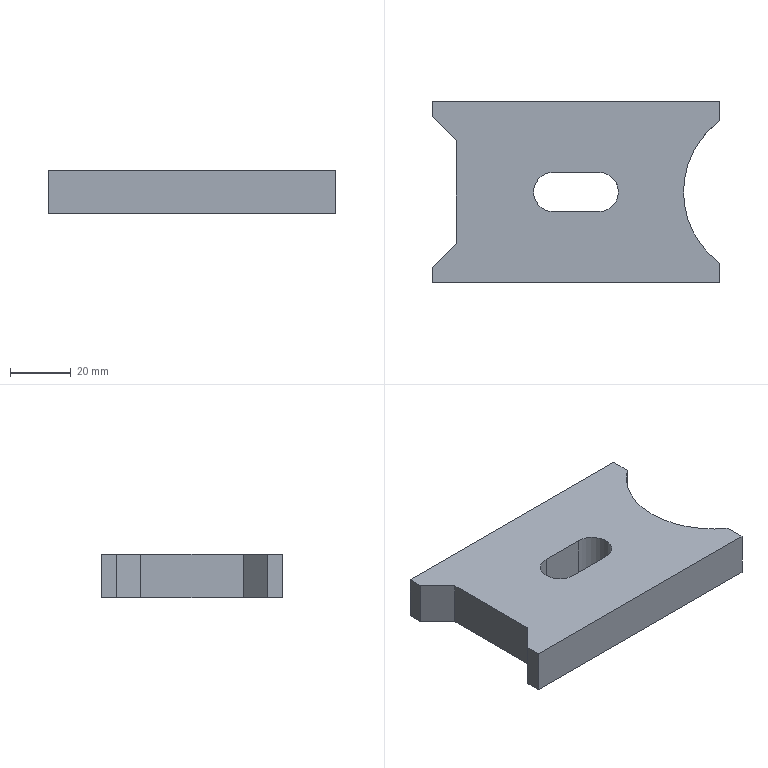Part | SolidWorks | features ICE 2, Shell 2, Extrusion 1 | 1 solid | 18 faces | box 95 x 60 x 14.5 mm | volume 67299 mm3 | plane 13 | cylinder 5 | commonest cylinder face diameters 13 x3 58.021 x2
STEP:
#1=CARTESIAN_POINT('',(47.5,23.5,14.5));
#2=VERTEX_POINT('',#1);
#3=CARTESIAN_POINT('',(35.5,0.,14.5));
#4=VERTEX_POINT('',#3);
#5=CARTESIAN_POINT('',(64.51,0.,14.5));
#6=DIRECTION('',(0.,0.,1.));
#7=DIRECTION('',(1.,0.,0.));
#8=AXIS2_PLACEMENT_3D('',#5,#6,#7);
#9=CIRCLE('',#8,29.01);
#10=EDGE_CURVE('',#2,#4,#9,.T.);
#11=ORIENTED_EDGE('',*,*,#10,.T.);
#12=CARTESIAN_POINT('',(35.5,0.,0.));
#13=VERTEX_POINT('',#12);
#14=CARTESIAN_POINT('',(35.5,0.,14.5));
#15=DIRECTION('',(0.,0.,-1.));
#16=VECTOR('',#15,1000.);
#17=LINE('',#14,#16);
#18=EDGE_CURVE('',#4,#13,#17,.T.);
#19=ORIENTED_EDGE('',*,*,#18,.T.);
#20=CARTESIAN_POINT('',(47.5,23.5,0.));
#21=VERTEX_POINT('',#20);
#22=CARTESIAN_POINT('',(64.51,0.,0.));
#23=DIRECTION('',(0.,0.,1.));
#24=DIRECTION('',(1.,0.,0.));
#25=AXIS2_PLACEMENT_3D('',#22,#23,#24);
#26=CIRCLE('',#25,29.01);
#27=EDGE_CURVE('',#21,#13,#26,.T.);
#28=ORIENTED_EDGE('',*,*,#27,.F.);
#29=CARTESIAN_POINT('',(47.5,23.5,14.5));
#30=DIRECTION('',(0.,0.,-1.));
#31=VECTOR('',#30,1000.);
#32=LINE('',#29,#31);
#33=EDGE_CURVE('',#2,#21,#32,.T.);
#34=ORIENTED_EDGE('',*,*,#33,.F.);
#35=EDGE_LOOP('',(#11,#19,#28,#34));
#36=FACE_OUTER_BOUND('',#35,.T.);
#37=CARTESIAN_POINT('',(64.51,0.,14.5));
#38=DIRECTION('',(0.,0.,-1.));
#39=DIRECTION('',(-1.,0.,0.));
#40=AXIS2_PLACEMENT_3D('',#37,#38,#39);
#41=CYLINDRICAL_SURFACE('',#40,29.01);
#42=ADVANCED_FACE('',(#36),#41,.F.);
#43=CARTESIAN_POINT('',(-14.,0.,14.5));
#44=VERTEX_POINT('',#43);
#45=CARTESIAN_POINT('',(-7.5,6.5,14.5));
#46=VERTEX_POINT('',#45);
#47=CARTESIAN_POINT('',(-7.5,0.,14.5));
#48=DIRECTION('',(0.,0.,-1.));
#49=DIRECTION('',(1.,0.,0.));
#50=AXIS2_PLACEMENT_3D('',#47,#48,#49);
#51=CIRCLE('',#50,6.5);
#52=EDGE_CURVE('',#44,#46,#51,.T.);
#53=ORIENTED_EDGE('',*,*,#52,.F.);
#54=CARTESIAN_POINT('',(-14.,0.,0.));
#55=VERTEX_POINT('',#54);
#56=CARTESIAN_POINT('',(-14.,0.,14.5));
#57=DIRECTION('',(0.,0.,-1.));
#58=VECTOR('',#57,1000.);
#59=LINE('',#56,#58);
#60=EDGE_CURVE('',#44,#55,#59,.T.);
#61=ORIENTED_EDGE('',*,*,#60,.T.);
#62=CARTESIAN_POINT('',(-7.5,6.5,0.));
#63=VERTEX_POINT('',#62);
#64=CARTESIAN_POINT('',(-7.5,0.,0.));
#65=DIRECTION('',(0.,0.,-1.));
#66=DIRECTION('',(1.,0.,0.));
#67=AXIS2_PLACEMENT_3D('',#64,#65,#66);
#68=CIRCLE('',#67,6.5);
#69=EDGE_CURVE('',#55,#63,#68,.T.);
#70=ORIENTED_EDGE('',*,*,#69,.T.);
#71=CARTESIAN_POINT('',(-7.5,6.5,14.5));
#72=DIRECTION('',(0.,0.,-1.));
#73=VECTOR('',#72,1000.);
#74=LINE('',#71,#73);
#75=EDGE_CURVE('',#46,#63,#74,.T.);
#76=ORIENTED_EDGE('',*,*,#75,.F.);
#77=EDGE_LOOP('',(#53,#61,#70,#76));
#78=FACE_OUTER_BOUND('',#77,.T.);
#79=CARTESIAN_POINT('',(-7.5,0.,14.5));
#80=DIRECTION('',(0.,0.,-1.));
#81=DIRECTION('',(-1.,0.,0.));
#82=AXIS2_PLACEMENT_3D('',#79,#80,#81);
#83=CYLINDRICAL_SURFACE('',#82,6.5);
#84=ADVANCED_FACE('',(#78),#83,.F.);
#85=CARTESIAN_POINT('',(-7.5,-6.5,0.));
#86=VERTEX_POINT('',#85);
#87=CARTESIAN_POINT('',(7.5,-6.5,0.));
#88=VERTEX_POINT('',#87);
#89=CARTESIAN_POINT('',(0.,-6.5,0.));
#90=DIRECTION('',(1.,0.,0.));
#91=VECTOR('',#90,1000.);
#92=LINE('',#89,#91);
#93=EDGE_CURVE('',#86,#88,#92,.T.);
#94=ORIENTED_EDGE('',*,*,#93,.F.);
#95=CARTESIAN_POINT('',(-7.5,-6.5,14.5));
#96=VERTEX_POINT('',#95);
#97=CARTESIAN_POINT('',(-7.5,-6.5,14.5));
#98=DIRECTION('',(0.,0.,-1.));
#99=VECTOR('',#98,1000.);
#100=LINE('',#97,#99);
#101=EDGE_CURVE('',#96,#86,#100,.T.);
#102=ORIENTED_EDGE('',*,*,#101,.F.);
#103=CARTESIAN_POINT('',(7.5,-6.5,14.5));
#104=VERTEX_POINT('',#103);
#105=CARTESIAN_POINT('',(0.,-6.5,14.5));
#106=DIRECTION('',(1.,0.,0.));
#107=VECTOR('',#106,1000.);
#108=LINE('',#105,#107);
#109=EDGE_CURVE('',#96,#104,#108,.T.);
#110=ORIENTED_EDGE('',*,*,#109,.T.);
#111=CARTESIAN_POINT('',(7.5,-6.5,14.5));
#112=DIRECTION('',(0.,0.,-1.));
#113=VECTOR('',#112,1000.);
#114=LINE('',#111,#113);
#115=EDGE_CURVE('',#104,#88,#114,.T.);
#116=ORIENTED_EDGE('',*,*,#115,.T.);
#117=EDGE_LOOP('',(#94,#102,#110,#116));
#118=FACE_OUTER_BOUND('',#117,.T.);
#119=CARTESIAN_POINT('',(0.,-6.5,14.5));
#120=DIRECTION('',(0.,1.,0.));
#121=DIRECTION('',(-1.,0.,0.));
#122=AXIS2_PLACEMENT_3D('',#119,#120,#121);
#123=PLANE('',#122);
#124=ADVANCED_FACE('',(#118),#123,.T.);
#125=ORIENTED_EDGE('',*,*,#60,.F.);
#126=CARTESIAN_POINT('',(-7.5,0.,14.5));
#127=DIRECTION('',(0.,0.,-1.));
#128=DIRECTION('',(1.,0.,0.));
#129=AXIS2_PLACEMENT_3D('',#126,#127,#128);
#130=CIRCLE('',#129,6.5);
#131=EDGE_CURVE('',#96,#44,#130,.T.);
#132=ORIENTED_EDGE('',*,*,#131,.F.);
#133=ORIENTED_EDGE('',*,*,#101,.T.);
#134=CARTESIAN_POINT('',(-7.5,0.,0.));
#135=DIRECTION('',(0.,0.,-1.));
#136=DIRECTION('',(1.,0.,0.));
#137=AXIS2_PLACEMENT_3D('',#134,#135,#136);
#138=CIRCLE('',#137,6.5);
#139=EDGE_CURVE('',#86,#55,#138,.T.);
#140=ORIENTED_EDGE('',*,*,#139,.T.);
#141=EDGE_LOOP('',(#125,#132,#133,#140));
#142=FACE_OUTER_BOUND('',#141,.T.);
#143=CARTESIAN_POINT('',(-7.5,0.,14.5));
#144=DIRECTION('',(0.,0.,-1.));
#145=DIRECTION('',(-1.,0.,0.));
#146=AXIS2_PLACEMENT_3D('',#143,#144,#145);
#147=CYLINDRICAL_SURFACE('',#146,6.5);
#148=ADVANCED_FACE('',(#142),#147,.F.);
#149=CARTESIAN_POINT('',(7.5,6.5,0.));
#150=VERTEX_POINT('',#149);
#151=CARTESIAN_POINT('',(0.,6.5,0.));
#152=DIRECTION('',(1.,0.,0.));
#153=VECTOR('',#152,1000.);
#154=LINE('',#151,#153);
#155=EDGE_CURVE('',#63,#150,#154,.T.);
#156=ORIENTED_EDGE('',*,*,#155,.T.);
#157=CARTESIAN_POINT('',(7.5,6.5,14.5));
#158=VERTEX_POINT('',#157);
#159=CARTESIAN_POINT('',(7.5,6.5,14.5));
#160=DIRECTION('',(0.,0.,-1.));
#161=VECTOR('',#160,1000.);
#162=LINE('',#159,#161);
#163=EDGE_CURVE('',#158,#150,#162,.T.);
#164=ORIENTED_EDGE('',*,*,#163,.F.);
#165=CARTESIAN_POINT('',(0.,6.5,14.5));
#166=DIRECTION('',(1.,0.,0.));
#167=VECTOR('',#166,1000.);
#168=LINE('',#165,#167);
#169=EDGE_CURVE('',#46,#158,#168,.T.);
#170=ORIENTED_EDGE('',*,*,#169,.F.);
#171=ORIENTED_EDGE('',*,*,#75,.T.);
#172=EDGE_LOOP('',(#156,#164,#170,#171));
#173=FACE_OUTER_BOUND('',#172,.T.);
#174=CARTESIAN_POINT('',(0.,6.5,14.5));
#175=DIRECTION('',(0.,1.,0.));
#176=DIRECTION('',(-1.,0.,0.));
#177=AXIS2_PLACEMENT_3D('',#174,#175,#176);
#178=PLANE('',#177);
#179=ADVANCED_FACE('',(#173),#178,.F.);
#180=ORIENTED_EDGE('',*,*,#18,.F.);
#181=CARTESIAN_POINT('',(47.5,-23.5,14.5));
#182=VERTEX_POINT('',#181);
#183=CARTESIAN_POINT('',(64.51,0.,14.5));
#184=DIRECTION('',(0.,0.,1.));
#185=DIRECTION('',(1.,0.,0.));
#186=AXIS2_PLACEMENT_3D('',#183,#184,#185);
#187=CIRCLE('',#186,29.01);
#188=EDGE_CURVE('',#4,#182,#187,.T.);
#189=ORIENTED_EDGE('',*,*,#188,.T.);
#190=CARTESIAN_POINT('',(47.5,-23.5,0.));
#191=VERTEX_POINT('',#190);
#192=CARTESIAN_POINT('',(47.5,-23.5,14.5));
#193=DIRECTION('',(0.,0.,-1.));
#194=VECTOR('',#193,1000.);
#195=LINE('',#192,#194);
#196=EDGE_CURVE('',#182,#191,#195,.T.);
#197=ORIENTED_EDGE('',*,*,#196,.T.);
#198=CARTESIAN_POINT('',(64.51,0.,0.));
#199=DIRECTION('',(0.,0.,1.));
#200=DIRECTION('',(1.,0.,0.));
#201=AXIS2_PLACEMENT_3D('',#198,#199,#200);
#202=CIRCLE('',#201,29.01);
#203=EDGE_CURVE('',#13,#191,#202,.T.);
#204=ORIENTED_EDGE('',*,*,#203,.F.);
#205=EDGE_LOOP('',(#180,#189,#197,#204));
#206=FACE_OUTER_BOUND('',#205,.T.);
#207=CARTESIAN_POINT('',(64.51,0.,14.5));
#208=DIRECTION('',(0.,0.,-1.));
#209=DIRECTION('',(-1.,0.,0.));
#210=AXIS2_PLACEMENT_3D('',#207,#208,#209);
#211=CYLINDRICAL_SURFACE('',#210,29.01);
#212=ADVANCED_FACE('',(#206),#211,.F.);
#213=CARTESIAN_POINT('',(47.5,30.,0.));
#214=VERTEX_POINT('',#213);
#215=CARTESIAN_POINT('',(47.5,0.,0.));
#216=DIRECTION('',(0.,-1.,0.));
#217=VECTOR('',#216,1000.);
#218=LINE('',#215,#217);
#219=EDGE_CURVE('',#214,#21,#218,.T.);
#220=ORIENTED_EDGE('',*,*,#219,.F.);
#221=CARTESIAN_POINT('',(47.5,30.,14.5));
#222=VERTEX_POINT('',#221);
#223=CARTESIAN_POINT('',(47.5,30.,14.5));
#224=DIRECTION('',(0.,0.,-1.));
#225=VECTOR('',#224,1000.);
#226=LINE('',#223,#225);
#227=EDGE_CURVE('',#222,#214,#226,.T.);
#228=ORIENTED_EDGE('',*,*,#227,.F.);
#229=CARTESIAN_POINT('',(47.5,0.,14.5));
#230=DIRECTION('',(0.,-1.,0.));
#231=VECTOR('',#230,1000.);
#232=LINE('',#229,#231);
#233=EDGE_CURVE('',#222,#2,#232,.T.);
#234=ORIENTED_EDGE('',*,*,#233,.T.);
#235=ORIENTED_EDGE('',*,*,#33,.T.);
#236=EDGE_LOOP('',(#220,#228,#234,#235));
#237=FACE_OUTER_BOUND('',#236,.T.);
#238=CARTESIAN_POINT('',(47.5,0.,14.5));
#239=DIRECTION('',(1.,0.,0.));
#240=DIRECTION('',(0.,1.,0.));
#241=AXIS2_PLACEMENT_3D('',#238,#239,#240);
#242=PLANE('',#241);
#243=ADVANCED_FACE('',(#237),#242,.T.);
#244=CARTESIAN_POINT('',(-47.5,30.,0.));
#245=VERTEX_POINT('',#244);
#246=CARTESIAN_POINT('',(0.,30.,0.));
#247=DIRECTION('',(1.,0.,0.));
#248=VECTOR('',#247,1000.);
#249=LINE('',#246,#248);
#250=EDGE_CURVE('',#245,#214,#249,.T.);
#251=ORIENTED_EDGE('',*,*,#250,.F.);
#252=CARTESIAN_POINT('',(-47.5,30.,14.5));
#253=VERTEX_POINT('',#252);
#254=CARTESIAN_POINT('',(-47.5,30.,14.5));
#255=DIRECTION('',(0.,0.,-1.));
#256=VECTOR('',#255,1000.);
#257=LINE('',#254,#256);
#258=EDGE_CURVE('',#253,#245,#257,.T.);
#259=ORIENTED_EDGE('',*,*,#258,.F.);
#260=CARTESIAN_POINT('',(0.,30.,14.5));
#261=DIRECTION('',(1.,0.,0.));
#262=VECTOR('',#261,1000.);
#263=LINE('',#260,#262);
#264=EDGE_CURVE('',#253,#222,#263,.T.);
#265=ORIENTED_EDGE('',*,*,#264,.T.);
#266=ORIENTED_EDGE('',*,*,#227,.T.);
#267=EDGE_LOOP('',(#251,#259,#265,#266));
#268=FACE_OUTER_BOUND('',#267,.T.);
#269=CARTESIAN_POINT('',(0.,30.,14.5));
#270=DIRECTION('',(0.,1.,0.));
#271=DIRECTION('',(0.,0.,1.));
#272=AXIS2_PLACEMENT_3D('',#269,#270,#271);
#273=PLANE('',#272);
#274=ADVANCED_FACE('',(#268),#273,.T.);
#275=CARTESIAN_POINT('',(-47.5,25.,0.));
#276=VERTEX_POINT('',#275);
#277=CARTESIAN_POINT('',(-47.5,0.,0.));
#278=DIRECTION('',(0.,-1.,0.));
#279=VECTOR('',#278,1000.);
#280=LINE('',#277,#279);
#281=EDGE_CURVE('',#245,#276,#280,.T.);
#282=ORIENTED_EDGE('',*,*,#281,.T.);
#283=CARTESIAN_POINT('',(-47.5,25.,14.5));
#284=VERTEX_POINT('',#283);
#285=CARTESIAN_POINT('',(-47.5,25.,14.5));
#286=DIRECTION('',(0.,0.,-1.));
#287=VECTOR('',#286,1000.);
#288=LINE('',#285,#287);
#289=EDGE_CURVE('',#284,#276,#288,.T.);
#290=ORIENTED_EDGE('',*,*,#289,.F.);
#291=CARTESIAN_POINT('',(-47.5,0.,14.5));
#292=DIRECTION('',(0.,-1.,0.));
#293=VECTOR('',#292,1000.);
#294=LINE('',#291,#293);
#295=EDGE_CURVE('',#253,#284,#294,.T.);
#296=ORIENTED_EDGE('',*,*,#295,.F.);
#297=ORIENTED_EDGE('',*,*,#258,.T.);
#298=EDGE_LOOP('',(#282,#290,#296,#297));
#299=FACE_OUTER_BOUND('',#298,.T.);
#300=CARTESIAN_POINT('',(-47.5,0.,14.5));
#301=DIRECTION('',(1.,0.,0.));
#302=DIRECTION('',(0.,0.,-1.));
#303=AXIS2_PLACEMENT_3D('',#300,#301,#302);
#304=PLANE('',#303);
#305=ADVANCED_FACE('',(#299),#304,.F.);
#306=CARTESIAN_POINT('',(-39.5,17.,0.));
#307=VERTEX_POINT('',#306);
#308=CARTESIAN_POINT('',(-11.25,-11.25,0.));
#309=DIRECTION('',(0.7071,-0.7071,0.));
#310=VECTOR('',#309,1000.);
#311=LINE('',#308,#310);
#312=EDGE_CURVE('',#276,#307,#311,.T.);
#313=ORIENTED_EDGE('',*,*,#312,.T.);
#314=CARTESIAN_POINT('',(-39.5,17.,14.5));
#315=VERTEX_POINT('',#314);
#316=CARTESIAN_POINT('',(-39.5,17.,14.5));
#317=DIRECTION('',(0.,0.,-1.));
#318=VECTOR('',#317,1000.);
#319=LINE('',#316,#318);
#320=EDGE_CURVE('',#315,#307,#319,.T.);
#321=ORIENTED_EDGE('',*,*,#320,.F.);
#322=CARTESIAN_POINT('',(-11.25,-11.25,14.5));
#323=DIRECTION('',(0.7071,-0.7071,0.));
#324=VECTOR('',#323,1000.);
#325=LINE('',#322,#324);
#326=EDGE_CURVE('',#284,#315,#325,.T.);
#327=ORIENTED_EDGE('',*,*,#326,.F.);
#328=ORIENTED_EDGE('',*,*,#289,.T.);
#329=EDGE_LOOP('',(#313,#321,#327,#328));
#330=FACE_OUTER_BOUND('',#329,.T.);
#331=CARTESIAN_POINT('',(-11.25,-11.25,14.5));
#332=DIRECTION('',(0.7071,0.7071,0.));
#333=DIRECTION('',(-0.7071,0.7071,0.));
#334=AXIS2_PLACEMENT_3D('',#331,#332,#333);
#335=PLANE('',#334);
#336=ADVANCED_FACE('',(#330),#335,.F.);
#337=CARTESIAN_POINT('',(-39.5,-17.,0.));
#338=VERTEX_POINT('',#337);
#339=CARTESIAN_POINT('',(-39.5,0.,0.));
#340=DIRECTION('',(0.,-1.,0.));
#341=VECTOR('',#340,1000.);
#342=LINE('',#339,#341);
#343=EDGE_CURVE('',#307,#338,#342,.T.);
#344=ORIENTED_EDGE('',*,*,#343,.T.);
#345=CARTESIAN_POINT('',(-39.5,-17.,14.5));
#346=VERTEX_POINT('',#345);
#347=CARTESIAN_POINT('',(-39.5,-17.,14.5));
#348=DIRECTION('',(0.,0.,-1.));
#349=VECTOR('',#348,1000.);
#350=LINE('',#347,#349);
#351=EDGE_CURVE('',#346,#338,#350,.T.);
#352=ORIENTED_EDGE('',*,*,#351,.F.);
#353=CARTESIAN_POINT('',(-39.5,0.,14.5));
#354=DIRECTION('',(0.,-1.,0.));
#355=VECTOR('',#354,1000.);
#356=LINE('',#353,#355);
#357=EDGE_CURVE('',#315,#346,#356,.T.);
#358=ORIENTED_EDGE('',*,*,#357,.F.);
#359=ORIENTED_EDGE('',*,*,#320,.T.);
#360=EDGE_LOOP('',(#344,#352,#358,#359));
#361=FACE_OUTER_BOUND('',#360,.T.);
#362=CARTESIAN_POINT('',(-39.5,0.,14.5));
#363=DIRECTION('',(1.,0.,0.));
#364=DIRECTION('',(0.,0.,-1.));
#365=AXIS2_PLACEMENT_3D('',#362,#363,#364);
#366=PLANE('',#365);
#367=ADVANCED_FACE('',(#361),#366,.F.);
#368=CARTESIAN_POINT('',(-47.5,-25.,0.));
#369=VERTEX_POINT('',#368);
#370=CARTESIAN_POINT('',(-11.25,11.25,0.));
#371=DIRECTION('',(0.7071,0.7071,0.));
#372=VECTOR('',#371,1000.);
#373=LINE('',#370,#372);
#374=EDGE_CURVE('',#369,#338,#373,.T.);
#375=ORIENTED_EDGE('',*,*,#374,.F.);
#376=CARTESIAN_POINT('',(-47.5,-25.,14.5));
#377=VERTEX_POINT('',#376);
#378=CARTESIAN_POINT('',(-47.5,-25.,14.5));
#379=DIRECTION('',(0.,0.,-1.));
#380=VECTOR('',#379,1000.);
#381=LINE('',#378,#380);
#382=EDGE_CURVE('',#377,#369,#381,.T.);
#383=ORIENTED_EDGE('',*,*,#382,.F.);
#384=CARTESIAN_POINT('',(-11.25,11.25,14.5));
#385=DIRECTION('',(0.7071,0.7071,0.));
#386=VECTOR('',#385,1000.);
#387=LINE('',#384,#386);
#388=EDGE_CURVE('',#377,#346,#387,.T.);
#389=ORIENTED_EDGE('',*,*,#388,.T.);
#390=ORIENTED_EDGE('',*,*,#351,.T.);
#391=EDGE_LOOP('',(#375,#383,#389,#390));
#392=FACE_OUTER_BOUND('',#391,.T.);
#393=CARTESIAN_POINT('',(-11.25,11.25,14.5));
#394=DIRECTION('',(-0.7071,0.7071,0.));
#395=DIRECTION('',(-0.7071,-0.7071,0.));
#396=AXIS2_PLACEMENT_3D('',#393,#394,#395);
#397=PLANE('',#396);
#398=ADVANCED_FACE('',(#392),#397,.T.);
#399=CARTESIAN_POINT('',(-47.5,-30.,0.));
#400=VERTEX_POINT('',#399);
#401=CARTESIAN_POINT('',(-47.5,0.,0.));
#402=DIRECTION('',(0.,-1.,0.));
#403=VECTOR('',#402,1000.);
#404=LINE('',#401,#403);
#405=EDGE_CURVE('',#369,#400,#404,.T.);
#406=ORIENTED_EDGE('',*,*,#405,.T.);
#407=CARTESIAN_POINT('',(-47.5,-30.,14.5));
#408=VERTEX_POINT('',#407);
#409=CARTESIAN_POINT('',(-47.5,-30.,14.5));
#410=DIRECTION('',(0.,0.,-1.));
#411=VECTOR('',#410,1000.);
#412=LINE('',#409,#411);
#413=EDGE_CURVE('',#408,#400,#412,.T.);
#414=ORIENTED_EDGE('',*,*,#413,.F.);
#415=CARTESIAN_POINT('',(-47.5,0.,14.5));
#416=DIRECTION('',(0.,-1.,0.));
#417=VECTOR('',#416,1000.);
#418=LINE('',#415,#417);
#419=EDGE_CURVE('',#377,#408,#418,.T.);
#420=ORIENTED_EDGE('',*,*,#419,.F.);
#421=ORIENTED_EDGE('',*,*,#382,.T.);
#422=EDGE_LOOP('',(#406,#414,#420,#421));
#423=FACE_OUTER_BOUND('',#422,.T.);
#424=CARTESIAN_POINT('',(-47.5,0.,14.5));
#425=DIRECTION('',(1.,0.,0.));
#426=DIRECTION('',(0.,1.,0.));
#427=AXIS2_PLACEMENT_3D('',#424,#425,#426);
#428=PLANE('',#427);
#429=ADVANCED_FACE('',(#423),#428,.F.);
#430=CARTESIAN_POINT('',(47.5,-30.,0.));
#431=VERTEX_POINT('',#430);
#432=CARTESIAN_POINT('',(0.,-30.,0.));
#433=DIRECTION('',(1.,0.,0.));
#434=VECTOR('',#433,1000.);
#435=LINE('',#432,#434);
#436=EDGE_CURVE('',#400,#431,#435,.T.);
#437=ORIENTED_EDGE('',*,*,#436,.T.);
#438=CARTESIAN_POINT('',(47.5,-30.,14.5));
#439=VERTEX_POINT('',#438);
#440=CARTESIAN_POINT('',(47.5,-30.,14.5));
#441=DIRECTION('',(0.,0.,-1.));
#442=VECTOR('',#441,1000.);
#443=LINE('',#440,#442);
#444=EDGE_CURVE('',#439,#431,#443,.T.);
#445=ORIENTED_EDGE('',*,*,#444,.F.);
#446=CARTESIAN_POINT('',(0.,-30.,14.5));
#447=DIRECTION('',(1.,0.,0.));
#448=VECTOR('',#447,1000.);
#449=LINE('',#446,#448);
#450=EDGE_CURVE('',#408,#439,#449,.T.);
#451=ORIENTED_EDGE('',*,*,#450,.F.);
#452=ORIENTED_EDGE('',*,*,#413,.T.);
#453=EDGE_LOOP('',(#437,#445,#451,#452));
#454=FACE_OUTER_BOUND('',#453,.T.);
#455=CARTESIAN_POINT('',(0.,-30.,14.5));
#456=DIRECTION('',(0.,1.,0.));
#457=DIRECTION('',(0.,0.,1.));
#458=AXIS2_PLACEMENT_3D('',#455,#456,#457);
#459=PLANE('',#458);
#460=ADVANCED_FACE('',(#454),#459,.F.);
#461=CARTESIAN_POINT('',(47.5,0.,0.));
#462=DIRECTION('',(0.,-1.,0.));
#463=VECTOR('',#462,1000.);
#464=LINE('',#461,#463);
#465=EDGE_CURVE('',#191,#431,#464,.T.);
#466=ORIENTED_EDGE('',*,*,#465,.F.);
#467=ORIENTED_EDGE('',*,*,#196,.F.);
#468=CARTESIAN_POINT('',(47.5,0.,14.5));
#469=DIRECTION('',(0.,-1.,0.));
#470=VECTOR('',#469,1000.);
#471=LINE('',#468,#470);
#472=EDGE_CURVE('',#182,#439,#471,.T.);
#473=ORIENTED_EDGE('',*,*,#472,.T.);
#474=ORIENTED_EDGE('',*,*,#444,.T.);
#475=EDGE_LOOP('',(#466,#467,#473,#474));
#476=FACE_OUTER_BOUND('',#475,.T.);
#477=CARTESIAN_POINT('',(47.5,0.,14.5));
#478=DIRECTION('',(1.,0.,0.));
#479=DIRECTION('',(0.,1.,0.));
#480=AXIS2_PLACEMENT_3D('',#477,#478,#479);
#481=PLANE('',#480);
#482=ADVANCED_FACE('',(#476),#481,.T.);
#483=CARTESIAN_POINT('',(7.5,0.,0.));
#484=DIRECTION('',(0.,0.,1.));
#485=DIRECTION('',(1.,0.,0.));
#486=AXIS2_PLACEMENT_3D('',#483,#484,#485);
#487=CIRCLE('',#486,6.5);
#488=EDGE_CURVE('',#88,#150,#487,.T.);
#489=ORIENTED_EDGE('',*,*,#488,.F.);
#490=ORIENTED_EDGE('',*,*,#115,.F.);
#491=CARTESIAN_POINT('',(7.5,0.,14.5));
#492=DIRECTION('',(0.,0.,1.));
#493=DIRECTION('',(1.,0.,0.));
#494=AXIS2_PLACEMENT_3D('',#491,#492,#493);
#495=CIRCLE('',#494,6.5);
#496=EDGE_CURVE('',#104,#158,#495,.T.);
#497=ORIENTED_EDGE('',*,*,#496,.T.);
#498=ORIENTED_EDGE('',*,*,#163,.T.);
#499=EDGE_LOOP('',(#489,#490,#497,#498));
#500=FACE_OUTER_BOUND('',#499,.T.);
#501=CARTESIAN_POINT('',(7.5,0.,14.5));
#502=DIRECTION('',(0.,0.,-1.));
#503=DIRECTION('',(-1.,0.,0.));
#504=AXIS2_PLACEMENT_3D('',#501,#502,#503);
#505=CYLINDRICAL_SURFACE('',#504,6.5);
#506=ADVANCED_FACE('',(#500),#505,.F.);
#507=ORIENTED_EDGE('',*,*,#10,.F.);
#508=ORIENTED_EDGE('',*,*,#233,.F.);
#509=ORIENTED_EDGE('',*,*,#264,.F.);
#510=ORIENTED_EDGE('',*,*,#295,.T.);
#511=ORIENTED_EDGE('',*,*,#326,.T.);
#512=ORIENTED_EDGE('',*,*,#357,.T.);
#513=ORIENTED_EDGE('',*,*,#388,.F.);
#514=ORIENTED_EDGE('',*,*,#419,.T.);
#515=ORIENTED_EDGE('',*,*,#450,.T.);
#516=ORIENTED_EDGE('',*,*,#472,.F.);
#517=ORIENTED_EDGE('',*,*,#188,.F.);
#518=EDGE_LOOP('',(#507,#508,#509,#510,#511,#512,#513,#514,#515,#516,#517));
#519=FACE_OUTER_BOUND('',#518,.T.);
#520=ORIENTED_EDGE('',*,*,#109,.F.);
#521=ORIENTED_EDGE('',*,*,#131,.T.);
#522=ORIENTED_EDGE('',*,*,#52,.T.);
#523=ORIENTED_EDGE('',*,*,#169,.T.);
#524=ORIENTED_EDGE('',*,*,#496,.F.);
#525=EDGE_LOOP('',(#520,#521,#522,#523,#524));
#526=FACE_BOUND('',#525,.T.);
#527=CARTESIAN_POINT('',(0.,0.,14.5));
#528=DIRECTION('',(0.,0.,1.));
#529=DIRECTION('',(1.,0.,0.));
#530=AXIS2_PLACEMENT_3D('',#527,#528,#529);
#531=PLANE('',#530);
#532=ADVANCED_FACE('',(#519,#526),#531,.T.);
#533=ORIENTED_EDGE('',*,*,#27,.T.);
#534=ORIENTED_EDGE('',*,*,#203,.T.);
#535=ORIENTED_EDGE('',*,*,#465,.T.);
#536=ORIENTED_EDGE('',*,*,#436,.F.);
#537=ORIENTED_EDGE('',*,*,#405,.F.);
#538=ORIENTED_EDGE('',*,*,#374,.T.);
#539=ORIENTED_EDGE('',*,*,#343,.F.);
#540=ORIENTED_EDGE('',*,*,#312,.F.);
#541=ORIENTED_EDGE('',*,*,#281,.F.);
#542=ORIENTED_EDGE('',*,*,#250,.T.);
#543=ORIENTED_EDGE('',*,*,#219,.T.);
#544=EDGE_LOOP('',(#533,#534,#535,#536,#537,#538,#539,#540,#541,#542,#543));
#545=FACE_OUTER_BOUND('',#544,.T.);
#546=ORIENTED_EDGE('',*,*,#93,.T.);
#547=ORIENTED_EDGE('',*,*,#488,.T.);
#548=ORIENTED_EDGE('',*,*,#155,.F.);
#549=ORIENTED_EDGE('',*,*,#69,.F.);
#550=ORIENTED_EDGE('',*,*,#139,.F.);
#551=EDGE_LOOP('',(#546,#547,#548,#549,#550));
#552=FACE_BOUND('',#551,.T.);
#553=CARTESIAN_POINT('',(0.,0.,0.));
#554=DIRECTION('',(0.,0.,1.));
#555=DIRECTION('',(1.,0.,0.));
#556=AXIS2_PLACEMENT_3D('',#553,#554,#555);
#557=PLANE('',#556);
#558=ADVANCED_FACE('',(#545,#552),#557,.F.);
#559=CLOSED_SHELL('',(#42,#84,#124,#148,#179,#212,#243,#274,#305,#336,#367,#398,#429,#460,#482,#506,#532,#558));
#560=MANIFOLD_SOLID_BREP('',#559);
#561=CARTESIAN_POINT('',(0.,0.,0.));
#562=DIRECTION('',(0.,0.,1.));
#563=DIRECTION('',(1.,0.,0.));
#564=AXIS2_PLACEMENT_3D('',#561,#562,#563);
#565=(LENGTH_UNIT()NAMED_UNIT(*)SI_UNIT(.MILLI.,.METRE.));
#566=UNCERTAINTY_MEASURE_WITH_UNIT(LENGTH_MEASURE(0.00001),#565,'','');
#567=(NAMED_UNIT(*)PLANE_ANGLE_UNIT()SI_UNIT($,.RADIAN.));
#568=(NAMED_UNIT(*)SI_UNIT($,.STERADIAN.)SOLID_ANGLE_UNIT());
#569=(GEOMETRIC_REPRESENTATION_CONTEXT(3)GLOBAL_UNCERTAINTY_ASSIGNED_CONTEXT((#566))GLOBAL_UNIT_ASSIGNED_CONTEXT((#565,#567,#568))REPRESENTATION_CONTEXT('',''));
#570=ADVANCED_BREP_SHAPE_REPRESENTATION('',(#560,#564),#569);